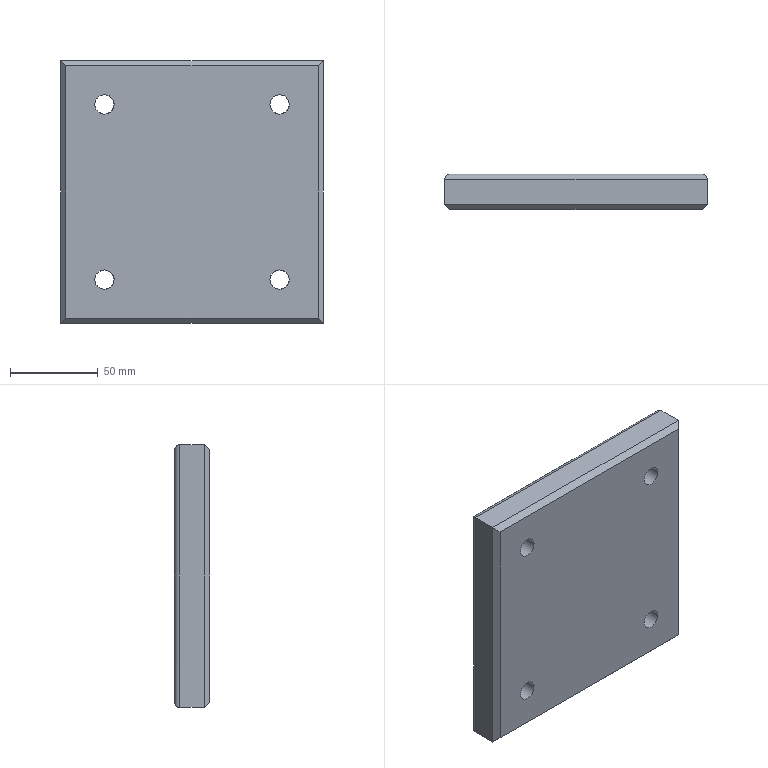Part | NX | features solid 2 | 1 solid | 26 faces | box 150 x 20 x 150 mm | volume 431601 mm3 | plane 14 | cylinder 12 | commonest cylinder face diameters 6 x4 11 x4 17.5 x4
STEP:
#1=CARTESIAN_POINT('',(1520.,643.,-110.));
#2=VERTEX_POINT('',#1);
#3=CARTESIAN_POINT('',(1520.,657.,-110.));
#4=VERTEX_POINT('',#3);
#5=CARTESIAN_POINT('',(1520.,640.,-110.));
#6=DIRECTION('',(0.,1.,0.));
#7=VECTOR('',#6,1000.);
#8=LINE('',#5,#7);
#9=EDGE_CURVE('',#2,#4,#8,.T.);
#10=ORIENTED_EDGE('',*,*,#9,.F.);
#11=CARTESIAN_POINT('',(1520.,643.,-260.));
#12=VERTEX_POINT('',#11);
#13=CARTESIAN_POINT('',(1520.,643.,-230.));
#14=DIRECTION('',(0.,0.,-1.));
#15=VECTOR('',#14,1000.);
#16=LINE('',#13,#15);
#17=EDGE_CURVE('',#2,#12,#16,.T.);
#18=ORIENTED_EDGE('',*,*,#17,.T.);
#19=CARTESIAN_POINT('',(1520.,657.,-260.));
#20=VERTEX_POINT('',#19);
#21=CARTESIAN_POINT('',(1520.,640.,-260.));
#22=DIRECTION('',(0.,1.,0.));
#23=VECTOR('',#22,1000.);
#24=LINE('',#21,#23);
#25=EDGE_CURVE('',#12,#20,#24,.T.);
#26=ORIENTED_EDGE('',*,*,#25,.T.);
#27=CARTESIAN_POINT('',(1520.,657.,-130.));
#28=DIRECTION('',(0.,0.,1.));
#29=VECTOR('',#28,1000.);
#30=LINE('',#27,#29);
#31=EDGE_CURVE('',#20,#4,#30,.T.);
#32=ORIENTED_EDGE('',*,*,#31,.T.);
#33=EDGE_LOOP('',(#10,#18,#26,#32));
#34=FACE_BOUND('',#33,.T.);
#35=CARTESIAN_POINT('',(1520.,640.,-230.));
#36=DIRECTION('',(-1.,0.,0.));
#37=DIRECTION('',(0.,0.,-1.));
#38=AXIS2_PLACEMENT_3D('',#35,#36,#37);
#39=PLANE('',#38);
#40=ADVANCED_FACE('',(#34),#39,.F.);
#41=CARTESIAN_POINT('',(1370.,643.,-110.));
#42=VERTEX_POINT('',#41);
#43=CARTESIAN_POINT('',(1370.,657.,-110.));
#44=VERTEX_POINT('',#43);
#45=CARTESIAN_POINT('',(1370.,640.,-110.));
#46=DIRECTION('',(0.,1.,0.));
#47=VECTOR('',#46,1000.);
#48=LINE('',#45,#47);
#49=EDGE_CURVE('',#42,#44,#48,.T.);
#50=ORIENTED_EDGE('',*,*,#49,.F.);
#51=CARTESIAN_POINT('',(1470.,643.,-110.));
#52=DIRECTION('',(1.,0.,0.));
#53=VECTOR('',#52,1000.);
#54=LINE('',#51,#53);
#55=EDGE_CURVE('',#42,#2,#54,.T.);
#56=ORIENTED_EDGE('',*,*,#55,.T.);
#57=ORIENTED_EDGE('',*,*,#9,.T.);
#58=CARTESIAN_POINT('',(1370.,657.,-110.));
#59=DIRECTION('',(-1.,0.,0.));
#60=VECTOR('',#59,1000.);
#61=LINE('',#58,#60);
#62=EDGE_CURVE('',#4,#44,#61,.T.);
#63=ORIENTED_EDGE('',*,*,#62,.T.);
#64=EDGE_LOOP('',(#50,#56,#57,#63));
#65=FACE_BOUND('',#64,.T.);
#66=CARTESIAN_POINT('',(1470.,640.,-110.));
#67=DIRECTION('',(0.,0.,-1.));
#68=DIRECTION('',(1.,0.,0.));
#69=AXIS2_PLACEMENT_3D('',#66,#67,#68);
#70=PLANE('',#69);
#71=ADVANCED_FACE('',(#65),#70,.F.);
#72=CARTESIAN_POINT('',(1370.,643.,-260.));
#73=VERTEX_POINT('',#72);
#74=CARTESIAN_POINT('',(1370.,657.,-260.));
#75=VERTEX_POINT('',#74);
#76=CARTESIAN_POINT('',(1370.,640.,-260.));
#77=DIRECTION('',(0.,1.,0.));
#78=VECTOR('',#77,1000.);
#79=LINE('',#76,#78);
#80=EDGE_CURVE('',#73,#75,#79,.T.);
#81=ORIENTED_EDGE('',*,*,#80,.F.);
#82=CARTESIAN_POINT('',(1370.,643.,-130.));
#83=DIRECTION('',(0.,0.,1.));
#84=VECTOR('',#83,1000.);
#85=LINE('',#82,#84);
#86=EDGE_CURVE('',#73,#42,#85,.T.);
#87=ORIENTED_EDGE('',*,*,#86,.T.);
#88=ORIENTED_EDGE('',*,*,#49,.T.);
#89=CARTESIAN_POINT('',(1370.,657.,-230.));
#90=DIRECTION('',(0.,0.,-1.));
#91=VECTOR('',#90,1000.);
#92=LINE('',#89,#91);
#93=EDGE_CURVE('',#44,#75,#92,.T.);
#94=ORIENTED_EDGE('',*,*,#93,.T.);
#95=EDGE_LOOP('',(#81,#87,#88,#94));
#96=FACE_BOUND('',#95,.T.);
#97=CARTESIAN_POINT('',(1370.,640.,-130.));
#98=DIRECTION('',(1.,0.,0.));
#99=DIRECTION('',(0.,-1.,0.));
#100=AXIS2_PLACEMENT_3D('',#97,#98,#99);
#101=PLANE('',#100);
#102=ADVANCED_FACE('',(#96),#101,.F.);
#103=ORIENTED_EDGE('',*,*,#25,.F.);
#104=CARTESIAN_POINT('',(1370.,643.,-260.));
#105=DIRECTION('',(-1.,0.,0.));
#106=VECTOR('',#105,1000.);
#107=LINE('',#104,#106);
#108=EDGE_CURVE('',#12,#73,#107,.T.);
#109=ORIENTED_EDGE('',*,*,#108,.T.);
#110=ORIENTED_EDGE('',*,*,#80,.T.);
#111=CARTESIAN_POINT('',(1470.,657.,-260.));
#112=DIRECTION('',(1.,0.,0.));
#113=VECTOR('',#112,1000.);
#114=LINE('',#111,#113);
#115=EDGE_CURVE('',#75,#20,#114,.T.);
#116=ORIENTED_EDGE('',*,*,#115,.T.);
#117=EDGE_LOOP('',(#103,#109,#110,#116));
#118=FACE_BOUND('',#117,.T.);
#119=CARTESIAN_POINT('',(1370.,640.,-260.));
#120=DIRECTION('',(0.,0.,1.));
#121=DIRECTION('',(-1.,0.,0.));
#122=AXIS2_PLACEMENT_3D('',#119,#120,#121);
#123=PLANE('',#122);
#124=ADVANCED_FACE('',(#118),#123,.F.);
#125=CARTESIAN_POINT('',(1517.,640.,-113.));
#126=VERTEX_POINT('',#125);
#127=CARTESIAN_POINT('',(1373.,640.,-113.));
#128=VERTEX_POINT('',#127);
#129=CARTESIAN_POINT('',(1470.,640.,-113.));
#130=DIRECTION('',(1.,0.,0.));
#131=VECTOR('',#130,1000.);
#132=LINE('',#129,#131);
#133=EDGE_CURVE('',#126,#128,#132,.F.);
#134=ORIENTED_EDGE('',*,*,#133,.T.);
#135=CARTESIAN_POINT('',(1373.,640.,-257.));
#136=VERTEX_POINT('',#135);
#137=CARTESIAN_POINT('',(1373.,640.,-230.));
#138=DIRECTION('',(0.,0.,-1.));
#139=VECTOR('',#138,1000.);
#140=LINE('',#137,#139);
#141=EDGE_CURVE('',#128,#136,#140,.T.);
#142=ORIENTED_EDGE('',*,*,#141,.T.);
#143=CARTESIAN_POINT('',(1517.,640.,-257.));
#144=VERTEX_POINT('',#143);
#145=CARTESIAN_POINT('',(1470.,640.,-257.));
#146=DIRECTION('',(-1.,0.,0.));
#147=VECTOR('',#146,1000.);
#148=LINE('',#145,#147);
#149=EDGE_CURVE('',#136,#144,#148,.F.);
#150=ORIENTED_EDGE('',*,*,#149,.T.);
#151=CARTESIAN_POINT('',(1517.,640.,-230.));
#152=DIRECTION('',(0.,0.,-1.));
#153=VECTOR('',#152,1000.);
#154=LINE('',#151,#153);
#155=EDGE_CURVE('',#144,#126,#154,.F.);
#156=ORIENTED_EDGE('',*,*,#155,.T.);
#157=EDGE_LOOP('',(#134,#142,#150,#156));
#158=FACE_BOUND('',#157,.T.);
#159=CARTESIAN_POINT('',(1395.,640.,-129.5));
#160=VERTEX_POINT('',#159);
#161=CARTESIAN_POINT('',(1395.,640.,-135.));
#162=DIRECTION('',(0.,1.,0.));
#163=DIRECTION('',(0.,0.,1.));
#164=AXIS2_PLACEMENT_3D('',#161,#162,#163);
#165=CIRCLE('',#164,5.5);
#166=EDGE_CURVE('',#160,#160,#165,.T.);
#167=ORIENTED_EDGE('',*,*,#166,.T.);
#168=EDGE_LOOP('',(#167));
#169=FACE_BOUND('',#168,.T.);
#170=CARTESIAN_POINT('',(1395.,640.,-229.5));
#171=VERTEX_POINT('',#170);
#172=CARTESIAN_POINT('',(1395.,640.,-235.));
#173=DIRECTION('',(0.,-1.,0.));
#174=DIRECTION('',(0.,0.,1.));
#175=AXIS2_PLACEMENT_3D('',#172,#173,#174);
#176=CIRCLE('',#175,5.5);
#177=EDGE_CURVE('',#171,#171,#176,.F.);
#178=ORIENTED_EDGE('',*,*,#177,.T.);
#179=EDGE_LOOP('',(#178));
#180=FACE_BOUND('',#179,.T.);
#181=CARTESIAN_POINT('',(1495.,640.,-129.5));
#182=VERTEX_POINT('',#181);
#183=CARTESIAN_POINT('',(1495.,640.,-135.));
#184=DIRECTION('',(0.,1.,0.));
#185=DIRECTION('',(0.,0.,1.));
#186=AXIS2_PLACEMENT_3D('',#183,#184,#185);
#187=CIRCLE('',#186,5.5);
#188=EDGE_CURVE('',#182,#182,#187,.T.);
#189=ORIENTED_EDGE('',*,*,#188,.T.);
#190=EDGE_LOOP('',(#189));
#191=FACE_BOUND('',#190,.T.);
#192=CARTESIAN_POINT('',(1495.,640.,-229.5));
#193=VERTEX_POINT('',#192);
#194=CARTESIAN_POINT('',(1495.,640.,-235.));
#195=DIRECTION('',(0.,-1.,0.));
#196=DIRECTION('',(0.,0.,1.));
#197=AXIS2_PLACEMENT_3D('',#194,#195,#196);
#198=CIRCLE('',#197,5.5);
#199=EDGE_CURVE('',#193,#193,#198,.F.);
#200=ORIENTED_EDGE('',*,*,#199,.T.);
#201=EDGE_LOOP('',(#200));
#202=FACE_BOUND('',#201,.T.);
#203=CARTESIAN_POINT('',(1470.,640.,-230.));
#204=DIRECTION('',(0.,1.,0.));
#205=DIRECTION('',(1.,0.,0.));
#206=AXIS2_PLACEMENT_3D('',#203,#204,#205);
#207=PLANE('',#206);
#208=ADVANCED_FACE('',(#158,#169,#180,#191,#202),#207,.F.);
#209=CARTESIAN_POINT('',(1517.,660.,-113.));
#210=VERTEX_POINT('',#209);
#211=CARTESIAN_POINT('',(1517.,660.,-257.));
#212=VERTEX_POINT('',#211);
#213=CARTESIAN_POINT('',(1517.,660.,-230.));
#214=DIRECTION('',(0.,0.,-1.));
#215=VECTOR('',#214,1000.);
#216=LINE('',#213,#215);
#217=EDGE_CURVE('',#210,#212,#216,.T.);
#218=ORIENTED_EDGE('',*,*,#217,.T.);
#219=CARTESIAN_POINT('',(1373.,660.,-257.));
#220=VERTEX_POINT('',#219);
#221=CARTESIAN_POINT('',(1470.,660.,-257.));
#222=DIRECTION('',(-1.,0.,0.));
#223=VECTOR('',#222,1000.);
#224=LINE('',#221,#223);
#225=EDGE_CURVE('',#212,#220,#224,.T.);
#226=ORIENTED_EDGE('',*,*,#225,.T.);
#227=CARTESIAN_POINT('',(1373.,660.,-113.));
#228=VERTEX_POINT('',#227);
#229=CARTESIAN_POINT('',(1373.,660.,-130.));
#230=DIRECTION('',(0.,0.,-1.));
#231=VECTOR('',#230,1000.);
#232=LINE('',#229,#231);
#233=EDGE_CURVE('',#220,#228,#232,.F.);
#234=ORIENTED_EDGE('',*,*,#233,.T.);
#235=CARTESIAN_POINT('',(1470.,660.,-113.));
#236=DIRECTION('',(-1.,0.,0.));
#237=VECTOR('',#236,1000.);
#238=LINE('',#235,#237);
#239=EDGE_CURVE('',#228,#210,#238,.F.);
#240=ORIENTED_EDGE('',*,*,#239,.T.);
#241=EDGE_LOOP('',(#218,#226,#234,#240));
#242=FACE_BOUND('',#241,.T.);
#243=CARTESIAN_POINT('',(1395.,660.,-126.25));
#244=VERTEX_POINT('',#243);
#245=CARTESIAN_POINT('',(1395.,660.,-135.));
#246=DIRECTION('',(0.,1.,0.));
#247=DIRECTION('',(0.,0.,1.));
#248=AXIS2_PLACEMENT_3D('',#245,#246,#247);
#249=CIRCLE('',#248,8.75);
#250=EDGE_CURVE('',#244,#244,#249,.F.);
#251=ORIENTED_EDGE('',*,*,#250,.T.);
#252=EDGE_LOOP('',(#251));
#253=FACE_BOUND('',#252,.T.);
#254=CARTESIAN_POINT('',(1395.,660.,-226.25));
#255=VERTEX_POINT('',#254);
#256=CARTESIAN_POINT('',(1395.,660.,-235.));
#257=DIRECTION('',(0.,-1.,0.));
#258=DIRECTION('',(0.,0.,1.));
#259=AXIS2_PLACEMENT_3D('',#256,#257,#258);
#260=CIRCLE('',#259,8.75);
#261=EDGE_CURVE('',#255,#255,#260,.T.);
#262=ORIENTED_EDGE('',*,*,#261,.T.);
#263=EDGE_LOOP('',(#262));
#264=FACE_BOUND('',#263,.T.);
#265=CARTESIAN_POINT('',(1495.,660.,-126.25));
#266=VERTEX_POINT('',#265);
#267=CARTESIAN_POINT('',(1495.,660.,-135.));
#268=DIRECTION('',(0.,1.,0.));
#269=DIRECTION('',(0.,0.,1.));
#270=AXIS2_PLACEMENT_3D('',#267,#268,#269);
#271=CIRCLE('',#270,8.75);
#272=EDGE_CURVE('',#266,#266,#271,.F.);
#273=ORIENTED_EDGE('',*,*,#272,.T.);
#274=EDGE_LOOP('',(#273));
#275=FACE_BOUND('',#274,.T.);
#276=CARTESIAN_POINT('',(1495.,660.,-226.25));
#277=VERTEX_POINT('',#276);
#278=CARTESIAN_POINT('',(1495.,660.,-235.));
#279=DIRECTION('',(0.,-1.,0.));
#280=DIRECTION('',(0.,0.,1.));
#281=AXIS2_PLACEMENT_3D('',#278,#279,#280);
#282=CIRCLE('',#281,8.75);
#283=EDGE_CURVE('',#277,#277,#282,.T.);
#284=ORIENTED_EDGE('',*,*,#283,.T.);
#285=EDGE_LOOP('',(#284));
#286=FACE_BOUND('',#285,.T.);
#287=CARTESIAN_POINT('',(1470.,660.,-230.));
#288=DIRECTION('',(0.,1.,0.));
#289=DIRECTION('',(1.,0.,0.));
#290=AXIS2_PLACEMENT_3D('',#287,#288,#289);
#291=PLANE('',#290);
#292=ADVANCED_FACE('',(#242,#253,#264,#275,#286),#291,.T.);
#293=CARTESIAN_POINT('',(1489.5,648.,-235.));
#294=VERTEX_POINT('',#293);
#295=CARTESIAN_POINT('',(1495.,648.,-235.));
#296=DIRECTION('',(0.,-1.,0.));
#297=DIRECTION('',(-1.,0.,0.));
#298=AXIS2_PLACEMENT_3D('',#295,#296,#297);
#299=CIRCLE('',#298,5.5);
#300=EDGE_CURVE('',#294,#294,#299,.T.);
#301=ORIENTED_EDGE('',*,*,#300,.F.);
#302=EDGE_LOOP('',(#301));
#303=FACE_BOUND('',#302,.T.);
#304=ORIENTED_EDGE('',*,*,#199,.F.);
#305=EDGE_LOOP('',(#304));
#306=FACE_BOUND('',#305,.T.);
#307=CARTESIAN_POINT('',(1495.,610.,-235.));
#308=DIRECTION('',(0.,-1.,0.));
#309=DIRECTION('',(-1.,0.,0.));
#310=AXIS2_PLACEMENT_3D('',#307,#308,#309);
#311=CYLINDRICAL_SURFACE('',#310,5.5);
#312=ADVANCED_FACE('',(#303,#306),#311,.F.);
#313=ORIENTED_EDGE('',*,*,#300,.T.);
#314=EDGE_LOOP('',(#313));
#315=FACE_BOUND('',#314,.T.);
#316=CARTESIAN_POINT('',(1486.25,648.,-235.));
#317=VERTEX_POINT('',#316);
#318=CARTESIAN_POINT('',(1495.,648.,-235.));
#319=DIRECTION('',(0.,-1.,0.));
#320=DIRECTION('',(-1.,0.,0.));
#321=AXIS2_PLACEMENT_3D('',#318,#319,#320);
#322=CIRCLE('',#321,8.75);
#323=EDGE_CURVE('',#317,#317,#322,.T.);
#324=ORIENTED_EDGE('',*,*,#323,.F.);
#325=EDGE_LOOP('',(#324));
#326=FACE_BOUND('',#325,.T.);
#327=CARTESIAN_POINT('',(1495.,648.,-235.));
#328=DIRECTION('',(0.,-1.,0.));
#329=DIRECTION('',(-1.,0.,0.));
#330=AXIS2_PLACEMENT_3D('',#327,#328,#329);
#331=PLANE('',#330);
#332=ADVANCED_FACE('',(#315,#326),#331,.F.);
#333=ORIENTED_EDGE('',*,*,#323,.T.);
#334=EDGE_LOOP('',(#333));
#335=FACE_BOUND('',#334,.T.);
#336=ORIENTED_EDGE('',*,*,#283,.F.);
#337=EDGE_LOOP('',(#336));
#338=FACE_BOUND('',#337,.T.);
#339=CARTESIAN_POINT('',(1495.,660.,-235.));
#340=DIRECTION('',(0.,-1.,0.));
#341=DIRECTION('',(-1.,0.,0.));
#342=AXIS2_PLACEMENT_3D('',#339,#340,#341);
#343=CYLINDRICAL_SURFACE('',#342,8.75);
#344=ADVANCED_FACE('',(#335,#338),#343,.F.);
#345=CARTESIAN_POINT('',(1489.5,648.,-135.));
#346=VERTEX_POINT('',#345);
#347=CARTESIAN_POINT('',(1495.,648.,-135.));
#348=DIRECTION('',(0.,-1.,0.));
#349=DIRECTION('',(-1.,0.,0.));
#350=AXIS2_PLACEMENT_3D('',#347,#348,#349);
#351=CIRCLE('',#350,5.5);
#352=EDGE_CURVE('',#346,#346,#351,.T.);
#353=ORIENTED_EDGE('',*,*,#352,.F.);
#354=EDGE_LOOP('',(#353));
#355=FACE_BOUND('',#354,.T.);
#356=ORIENTED_EDGE('',*,*,#188,.F.);
#357=EDGE_LOOP('',(#356));
#358=FACE_BOUND('',#357,.T.);
#359=CARTESIAN_POINT('',(1495.,610.,-135.));
#360=DIRECTION('',(0.,-1.,0.));
#361=DIRECTION('',(-1.,0.,0.));
#362=AXIS2_PLACEMENT_3D('',#359,#360,#361);
#363=CYLINDRICAL_SURFACE('',#362,5.5);
#364=ADVANCED_FACE('',(#355,#358),#363,.F.);
#365=ORIENTED_EDGE('',*,*,#352,.T.);
#366=EDGE_LOOP('',(#365));
#367=FACE_BOUND('',#366,.T.);
#368=CARTESIAN_POINT('',(1486.25,648.,-135.));
#369=VERTEX_POINT('',#368);
#370=CARTESIAN_POINT('',(1495.,648.,-135.));
#371=DIRECTION('',(0.,-1.,0.));
#372=DIRECTION('',(-1.,0.,0.));
#373=AXIS2_PLACEMENT_3D('',#370,#371,#372);
#374=CIRCLE('',#373,8.75);
#375=EDGE_CURVE('',#369,#369,#374,.T.);
#376=ORIENTED_EDGE('',*,*,#375,.F.);
#377=EDGE_LOOP('',(#376));
#378=FACE_BOUND('',#377,.T.);
#379=CARTESIAN_POINT('',(1495.,648.,-135.));
#380=DIRECTION('',(0.,-1.,0.));
#381=DIRECTION('',(-1.,0.,0.));
#382=AXIS2_PLACEMENT_3D('',#379,#380,#381);
#383=PLANE('',#382);
#384=ADVANCED_FACE('',(#367,#378),#383,.F.);
#385=ORIENTED_EDGE('',*,*,#375,.T.);
#386=EDGE_LOOP('',(#385));
#387=FACE_BOUND('',#386,.T.);
#388=ORIENTED_EDGE('',*,*,#272,.F.);
#389=EDGE_LOOP('',(#388));
#390=FACE_BOUND('',#389,.T.);
#391=CARTESIAN_POINT('',(1495.,660.,-135.));
#392=DIRECTION('',(0.,-1.,0.));
#393=DIRECTION('',(-1.,0.,0.));
#394=AXIS2_PLACEMENT_3D('',#391,#392,#393);
#395=CYLINDRICAL_SURFACE('',#394,8.75);
#396=ADVANCED_FACE('',(#387,#390),#395,.F.);
#397=CARTESIAN_POINT('',(1389.5,648.,-235.));
#398=VERTEX_POINT('',#397);
#399=CARTESIAN_POINT('',(1395.,648.,-235.));
#400=DIRECTION('',(0.,-1.,0.));
#401=DIRECTION('',(-1.,0.,0.));
#402=AXIS2_PLACEMENT_3D('',#399,#400,#401);
#403=CIRCLE('',#402,5.5);
#404=EDGE_CURVE('',#398,#398,#403,.T.);
#405=ORIENTED_EDGE('',*,*,#404,.F.);
#406=EDGE_LOOP('',(#405));
#407=FACE_BOUND('',#406,.T.);
#408=ORIENTED_EDGE('',*,*,#177,.F.);
#409=EDGE_LOOP('',(#408));
#410=FACE_BOUND('',#409,.T.);
#411=CARTESIAN_POINT('',(1395.,610.,-235.));
#412=DIRECTION('',(0.,-1.,0.));
#413=DIRECTION('',(-1.,0.,0.));
#414=AXIS2_PLACEMENT_3D('',#411,#412,#413);
#415=CYLINDRICAL_SURFACE('',#414,5.5);
#416=ADVANCED_FACE('',(#407,#410),#415,.F.);
#417=ORIENTED_EDGE('',*,*,#404,.T.);
#418=EDGE_LOOP('',(#417));
#419=FACE_BOUND('',#418,.T.);
#420=CARTESIAN_POINT('',(1386.25,648.,-235.));
#421=VERTEX_POINT('',#420);
#422=CARTESIAN_POINT('',(1395.,648.,-235.));
#423=DIRECTION('',(0.,-1.,0.));
#424=DIRECTION('',(-1.,0.,0.));
#425=AXIS2_PLACEMENT_3D('',#422,#423,#424);
#426=CIRCLE('',#425,8.75);
#427=EDGE_CURVE('',#421,#421,#426,.T.);
#428=ORIENTED_EDGE('',*,*,#427,.F.);
#429=EDGE_LOOP('',(#428));
#430=FACE_BOUND('',#429,.T.);
#431=CARTESIAN_POINT('',(1395.,648.,-235.));
#432=DIRECTION('',(0.,-1.,0.));
#433=DIRECTION('',(-1.,0.,0.));
#434=AXIS2_PLACEMENT_3D('',#431,#432,#433);
#435=PLANE('',#434);
#436=ADVANCED_FACE('',(#419,#430),#435,.F.);
#437=ORIENTED_EDGE('',*,*,#427,.T.);
#438=EDGE_LOOP('',(#437));
#439=FACE_BOUND('',#438,.T.);
#440=ORIENTED_EDGE('',*,*,#261,.F.);
#441=EDGE_LOOP('',(#440));
#442=FACE_BOUND('',#441,.T.);
#443=CARTESIAN_POINT('',(1395.,660.,-235.));
#444=DIRECTION('',(0.,-1.,0.));
#445=DIRECTION('',(-1.,0.,0.));
#446=AXIS2_PLACEMENT_3D('',#443,#444,#445);
#447=CYLINDRICAL_SURFACE('',#446,8.75);
#448=ADVANCED_FACE('',(#439,#442),#447,.F.);
#449=CARTESIAN_POINT('',(1389.5,648.,-135.));
#450=VERTEX_POINT('',#449);
#451=CARTESIAN_POINT('',(1395.,648.,-135.));
#452=DIRECTION('',(0.,-1.,0.));
#453=DIRECTION('',(-1.,0.,0.));
#454=AXIS2_PLACEMENT_3D('',#451,#452,#453);
#455=CIRCLE('',#454,5.5);
#456=EDGE_CURVE('',#450,#450,#455,.T.);
#457=ORIENTED_EDGE('',*,*,#456,.F.);
#458=EDGE_LOOP('',(#457));
#459=FACE_BOUND('',#458,.T.);
#460=ORIENTED_EDGE('',*,*,#166,.F.);
#461=EDGE_LOOP('',(#460));
#462=FACE_BOUND('',#461,.T.);
#463=CARTESIAN_POINT('',(1395.,610.,-135.));
#464=DIRECTION('',(0.,-1.,0.));
#465=DIRECTION('',(-1.,0.,0.));
#466=AXIS2_PLACEMENT_3D('',#463,#464,#465);
#467=CYLINDRICAL_SURFACE('',#466,5.5);
#468=ADVANCED_FACE('',(#459,#462),#467,.F.);
#469=ORIENTED_EDGE('',*,*,#456,.T.);
#470=EDGE_LOOP('',(#469));
#471=FACE_BOUND('',#470,.T.);
#472=CARTESIAN_POINT('',(1386.25,648.,-135.));
#473=VERTEX_POINT('',#472);
#474=CARTESIAN_POINT('',(1395.,648.,-135.));
#475=DIRECTION('',(0.,-1.,0.));
#476=DIRECTION('',(-1.,0.,0.));
#477=AXIS2_PLACEMENT_3D('',#474,#475,#476);
#478=CIRCLE('',#477,8.75);
#479=EDGE_CURVE('',#473,#473,#478,.T.);
#480=ORIENTED_EDGE('',*,*,#479,.F.);
#481=EDGE_LOOP('',(#480));
#482=FACE_BOUND('',#481,.T.);
#483=CARTESIAN_POINT('',(1395.,648.,-135.));
#484=DIRECTION('',(0.,-1.,0.));
#485=DIRECTION('',(-1.,0.,0.));
#486=AXIS2_PLACEMENT_3D('',#483,#484,#485);
#487=PLANE('',#486);
#488=ADVANCED_FACE('',(#471,#482),#487,.F.);
#489=ORIENTED_EDGE('',*,*,#479,.T.);
#490=EDGE_LOOP('',(#489));
#491=FACE_BOUND('',#490,.T.);
#492=ORIENTED_EDGE('',*,*,#250,.F.);
#493=EDGE_LOOP('',(#492));
#494=FACE_BOUND('',#493,.T.);
#495=CARTESIAN_POINT('',(1395.,660.,-135.));
#496=DIRECTION('',(0.,-1.,0.));
#497=DIRECTION('',(-1.,0.,0.));
#498=AXIS2_PLACEMENT_3D('',#495,#496,#497);
#499=CYLINDRICAL_SURFACE('',#498,8.75);
#500=ADVANCED_FACE('',(#491,#494),#499,.F.);
#501=CARTESIAN_POINT('',(1517.,657.,-113.));
#502=DIRECTION('',(0.7071,0.,-0.7071));
#503=DIRECTION('',(-0.7071,0.,-0.7071));
#504=AXIS2_PLACEMENT_3D('',#501,#502,#503);
#505=ELLIPSE('',#504,4.243,3.);
#506=EDGE_CURVE('',#210,#4,#505,.T.);
#507=ORIENTED_EDGE('',*,*,#506,.F.);
#508=ORIENTED_EDGE('',*,*,#239,.F.);
#509=CARTESIAN_POINT('',(1373.,657.,-113.));
#510=DIRECTION('',(0.7071,0.,0.7071));
#511=DIRECTION('',(-0.7071,0.,0.7071));
#512=AXIS2_PLACEMENT_3D('',#509,#510,#511);
#513=ELLIPSE('',#512,4.243,3.);
#514=EDGE_CURVE('',#44,#228,#513,.F.);
#515=ORIENTED_EDGE('',*,*,#514,.F.);
#516=ORIENTED_EDGE('',*,*,#62,.F.);
#517=EDGE_LOOP('',(#507,#508,#515,#516));
#518=FACE_BOUND('',#517,.T.);
#519=CARTESIAN_POINT('',(1470.,657.,-113.));
#520=DIRECTION('',(1.,0.,0.));
#521=DIRECTION('',(0.,0.,1.));
#522=AXIS2_PLACEMENT_3D('',#519,#520,#521);
#523=CYLINDRICAL_SURFACE('',#522,3.);
#524=ADVANCED_FACE('',(#518),#523,.T.);
#525=ORIENTED_EDGE('',*,*,#514,.T.);
#526=ORIENTED_EDGE('',*,*,#233,.F.);
#527=CARTESIAN_POINT('',(1373.,657.,-257.));
#528=DIRECTION('',(0.7071,0.,-0.7071));
#529=DIRECTION('',(0.7071,0.,0.7071));
#530=AXIS2_PLACEMENT_3D('',#527,#528,#529);
#531=ELLIPSE('',#530,4.243,3.);
#532=EDGE_CURVE('',#75,#220,#531,.T.);
#533=ORIENTED_EDGE('',*,*,#532,.F.);
#534=ORIENTED_EDGE('',*,*,#93,.F.);
#535=EDGE_LOOP('',(#525,#526,#533,#534));
#536=FACE_BOUND('',#535,.T.);
#537=CARTESIAN_POINT('',(1373.,657.,-130.));
#538=DIRECTION('',(0.,0.,1.));
#539=DIRECTION('',(0.,1.,0.));
#540=AXIS2_PLACEMENT_3D('',#537,#538,#539);
#541=CYLINDRICAL_SURFACE('',#540,3.);
#542=ADVANCED_FACE('',(#536),#541,.T.);
#543=ORIENTED_EDGE('',*,*,#506,.T.);
#544=ORIENTED_EDGE('',*,*,#31,.F.);
#545=CARTESIAN_POINT('',(1517.,657.,-257.));
#546=DIRECTION('',(0.7071,0.,0.7071));
#547=DIRECTION('',(0.7071,0.,-0.7071));
#548=AXIS2_PLACEMENT_3D('',#545,#546,#547);
#549=ELLIPSE('',#548,4.243,3.);
#550=EDGE_CURVE('',#212,#20,#549,.F.);
#551=ORIENTED_EDGE('',*,*,#550,.F.);
#552=ORIENTED_EDGE('',*,*,#217,.F.);
#553=EDGE_LOOP('',(#543,#544,#551,#552));
#554=FACE_BOUND('',#553,.T.);
#555=CARTESIAN_POINT('',(1517.,657.,-230.));
#556=DIRECTION('',(0.,0.,-1.));
#557=DIRECTION('',(1.,0.,0.));
#558=AXIS2_PLACEMENT_3D('',#555,#556,#557);
#559=CYLINDRICAL_SURFACE('',#558,3.);
#560=ADVANCED_FACE('',(#554),#559,.T.);
#561=ORIENTED_EDGE('',*,*,#532,.T.);
#562=ORIENTED_EDGE('',*,*,#225,.F.);
#563=ORIENTED_EDGE('',*,*,#550,.T.);
#564=ORIENTED_EDGE('',*,*,#115,.F.);
#565=EDGE_LOOP('',(#561,#562,#563,#564));
#566=FACE_BOUND('',#565,.T.);
#567=CARTESIAN_POINT('',(1370.,657.,-257.));
#568=DIRECTION('',(-1.,0.,0.));
#569=DIRECTION('',(0.,0.,-1.));
#570=AXIS2_PLACEMENT_3D('',#567,#568,#569);
#571=CYLINDRICAL_SURFACE('',#570,3.);
#572=ADVANCED_FACE('',(#566),#571,.T.);
#573=CARTESIAN_POINT('',(1508.,631.,-248.));
#574=DIRECTION('',(-0.5774,-0.5774,0.5774));
#575=VECTOR('',#574,1000.);
#576=LINE('',#573,#575);
#577=EDGE_CURVE('',#12,#144,#576,.T.);
#578=ORIENTED_EDGE('',*,*,#577,.F.);
#579=ORIENTED_EDGE('',*,*,#17,.F.);
#580=CARTESIAN_POINT('',(1501.333,624.333,-128.667));
#581=DIRECTION('',(0.5774,0.5774,0.5774));
#582=VECTOR('',#581,1000.);
#583=LINE('',#580,#582);
#584=EDGE_CURVE('',#126,#2,#583,.T.);
#585=ORIENTED_EDGE('',*,*,#584,.F.);
#586=ORIENTED_EDGE('',*,*,#155,.F.);
#587=EDGE_LOOP('',(#578,#579,#585,#586));
#588=FACE_BOUND('',#587,.T.);
#589=CARTESIAN_POINT('',(1517.,640.,-230.));
#590=DIRECTION('',(-0.7071,0.7071,0.));
#591=DIRECTION('',(0.7071,0.7071,0.));
#592=AXIS2_PLACEMENT_3D('',#589,#590,#591);
#593=PLANE('',#592);
#594=ADVANCED_FACE('',(#588),#593,.F.);
#595=ORIENTED_EDGE('',*,*,#584,.T.);
#596=ORIENTED_EDGE('',*,*,#55,.F.);
#597=CARTESIAN_POINT('',(1412.,601.,-152.));
#598=DIRECTION('',(-0.5774,0.5774,0.5774));
#599=VECTOR('',#598,1000.);
#600=LINE('',#597,#599);
#601=EDGE_CURVE('',#128,#42,#600,.T.);
#602=ORIENTED_EDGE('',*,*,#601,.F.);
#603=ORIENTED_EDGE('',*,*,#133,.F.);
#604=EDGE_LOOP('',(#595,#596,#602,#603));
#605=FACE_BOUND('',#604,.T.);
#606=CARTESIAN_POINT('',(1470.,640.,-113.));
#607=DIRECTION('',(0.,0.7071,-0.7071));
#608=DIRECTION('',(0.,-0.7071,-0.7071));
#609=AXIS2_PLACEMENT_3D('',#606,#607,#608);
#610=PLANE('',#609);
#611=ADVANCED_FACE('',(#605),#610,.F.);
#612=ORIENTED_EDGE('',*,*,#577,.T.);
#613=ORIENTED_EDGE('',*,*,#149,.F.);
#614=CARTESIAN_POINT('',(1405.333,607.667,-224.667));
#615=DIRECTION('',(0.5774,-0.5774,0.5774));
#616=VECTOR('',#615,1000.);
#617=LINE('',#614,#616);
#618=EDGE_CURVE('',#73,#136,#617,.T.);
#619=ORIENTED_EDGE('',*,*,#618,.F.);
#620=ORIENTED_EDGE('',*,*,#108,.F.);
#621=EDGE_LOOP('',(#612,#613,#619,#620));
#622=FACE_BOUND('',#621,.T.);
#623=CARTESIAN_POINT('',(1470.,640.,-257.));
#624=DIRECTION('',(0.,0.7071,0.7071));
#625=DIRECTION('',(0.,0.7071,-0.7071));
#626=AXIS2_PLACEMENT_3D('',#623,#624,#625);
#627=PLANE('',#626);
#628=ADVANCED_FACE('',(#622),#627,.F.);
#629=ORIENTED_EDGE('',*,*,#601,.T.);
#630=ORIENTED_EDGE('',*,*,#86,.F.);
#631=ORIENTED_EDGE('',*,*,#618,.T.);
#632=ORIENTED_EDGE('',*,*,#141,.F.);
#633=EDGE_LOOP('',(#629,#630,#631,#632));
#634=FACE_BOUND('',#633,.T.);
#635=CARTESIAN_POINT('',(1373.,640.,-230.));
#636=DIRECTION('',(0.7071,0.7071,0.));
#637=DIRECTION('',(0.7071,-0.7071,0.));
#638=AXIS2_PLACEMENT_3D('',#635,#636,#637);
#639=PLANE('',#638);
#640=ADVANCED_FACE('',(#634),#639,.F.);
#641=CLOSED_SHELL('',(#40,#71,#102,#124,#208,#292,#312,#332,#344,#364,#384,#396,#416,#436,#448,#468,#488,#500,#524,#542,#560,#572,#594,#611,#628,#640));
#642=MANIFOLD_SOLID_BREP('',#641);
#643=(LENGTH_UNIT()NAMED_UNIT(*)SI_UNIT(.MILLI.,.METRE.));
#644=UNCERTAINTY_MEASURE_WITH_UNIT(LENGTH_MEASURE(0.00001),#643,'','');
#645=(NAMED_UNIT(*)PLANE_ANGLE_UNIT()SI_UNIT($,.RADIAN.));
#646=(NAMED_UNIT(*)SI_UNIT($,.STERADIAN.)SOLID_ANGLE_UNIT());
#647=(GEOMETRIC_REPRESENTATION_CONTEXT(3)GLOBAL_UNCERTAINTY_ASSIGNED_CONTEXT((#644))GLOBAL_UNIT_ASSIGNED_CONTEXT((#643,#645,#646))REPRESENTATION_CONTEXT('',''));
#648=ADVANCED_BREP_SHAPE_REPRESENTATION('',(#642),#647);